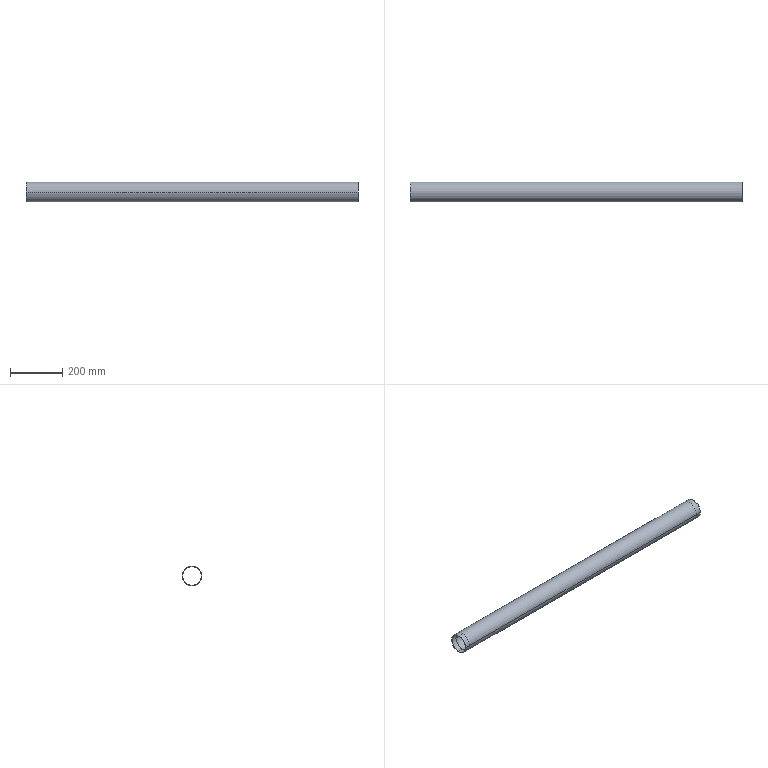Part | STEP file | DCV-000-001 | 1 solid | 12 faces | box 1270 x 76.3 x 76.3 mm | volume 923470 mm3 | cylinder 8 | plane 4 | commonest cylinder face diameters 72 x4 69.9 x2 76.3 x2
STEP:
#1=CARTESIAN_POINT('',(0.,0.,0.));
#2=DIRECTION('',(0.,0.,1.));
#3=DIRECTION('',(1.,0.,0.));
#4=AXIS2_PLACEMENT_3D('',#1,#2,#3);
#5=CARTESIAN_POINT('',(-635.,0.,36.));
#6=VERTEX_POINT('',#5);
#7=CARTESIAN_POINT('',(-614.,0.,36.));
#8=VERTEX_POINT('',#7);
#9=CARTESIAN_POINT('',(-635.,0.,36.));
#10=DIRECTION('',(1.,0.,0.));
#11=VECTOR('',#10,1.);
#12=LINE('',#9,#11);
#13=CARTESIAN_POINT('',(-635.,0.,0.));
#14=DIRECTION('',(1.,0.,0.));
#15=DIRECTION('',(0.,0.,1.));
#16=AXIS2_PLACEMENT_3D('',#13,#14,#15);
#17=CYLINDRICAL_SURFACE('',#16,36.);
#18=CARTESIAN_POINT('',(6.283,0.));
#19=DIRECTION('',(0.,1.));
#20=VECTOR('',#19,1.);
#21=LINE('',#18,#20);
#22=(GEOMETRIC_REPRESENTATION_CONTEXT(2)PARAMETRIC_REPRESENTATION_CONTEXT()REPRESENTATION_CONTEXT('',''));
#23=DEFINITIONAL_REPRESENTATION('',(#21),#22);
#24=PCURVE('',#17,#23);
#25=CARTESIAN_POINT('',(-635.,0.,0.));
#26=DIRECTION('',(1.,0.,0.));
#27=DIRECTION('',(0.,0.,1.));
#28=AXIS2_PLACEMENT_3D('',#25,#26,#27);
#29=CYLINDRICAL_SURFACE('',#28,36.);
#30=CARTESIAN_POINT('',(0.,0.));
#31=DIRECTION('',(0.,1.));
#32=VECTOR('',#31,1.);
#33=LINE('',#30,#32);
#34=(GEOMETRIC_REPRESENTATION_CONTEXT(2)PARAMETRIC_REPRESENTATION_CONTEXT()REPRESENTATION_CONTEXT('',''));
#35=DEFINITIONAL_REPRESENTATION('',(#33),#34);
#36=PCURVE('',#29,#35);
#37=SURFACE_CURVE('',#12,(#24,#36),.PCURVE_S1.);
#38=EDGE_CURVE('',#6,#8,#37,.T.);
#39=ORIENTED_EDGE('',*,*,#38,.T.);
#40=CARTESIAN_POINT('',(-614.,0.,-36.));
#41=VERTEX_POINT('',#40);
#42=CARTESIAN_POINT('',(-614.,0.,0.));
#43=DIRECTION('',(1.,0.,0.));
#44=DIRECTION('',(0.,0.,1.));
#45=AXIS2_PLACEMENT_3D('',#42,#43,#44);
#46=CIRCLE('',#45,36.);
#47=CARTESIAN_POINT('',(0.,21.));
#48=DIRECTION('',(1.,0.));
#49=VECTOR('',#48,1.);
#50=LINE('',#47,#49);
#51=(GEOMETRIC_REPRESENTATION_CONTEXT(2)PARAMETRIC_REPRESENTATION_CONTEXT()REPRESENTATION_CONTEXT('',''));
#52=DEFINITIONAL_REPRESENTATION('',(#50),#51);
#53=PCURVE('',#17,#52);
#54=CARTESIAN_POINT('',(-614.,0.,0.));
#55=DIRECTION('',(-1.,0.,0.));
#56=DIRECTION('',(0.,0.,1.));
#57=AXIS2_PLACEMENT_3D('',#54,#55,#56);
#58=PLANE('',#57);
#59=CARTESIAN_POINT('',(36.,0.));
#60=CARTESIAN_POINT('',(36.,-62.354));
#61=CARTESIAN_POINT('',(-18.,-31.177));
#62=CARTESIAN_POINT('',(-72.,0.));
#63=CARTESIAN_POINT('',(-18.,31.177));
#64=CARTESIAN_POINT('',(36.,62.354));
#65=CARTESIAN_POINT('',(36.,0.));
#66=(BOUNDED_CURVE()B_SPLINE_CURVE(2,(#59,#60,#61,#62,#63,#64,#65),.UNSPECIFIED.,.T.,.F.)B_SPLINE_CURVE_WITH_KNOTS((1,2,2,2,2,1),(-2.094,0.,2.094,4.189,6.283,8.378),.UNSPECIFIED.)CURVE()GEOMETRIC_REPRESENTATION_ITEM()RATIONAL_B_SPLINE_CURVE((1.,0.5,1.,0.5,1.,0.5,1.))REPRESENTATION_ITEM(''));
#67=(GEOMETRIC_REPRESENTATION_CONTEXT(2)PARAMETRIC_REPRESENTATION_CONTEXT()REPRESENTATION_CONTEXT('',''));
#68=DEFINITIONAL_REPRESENTATION('',(#66),#67);
#69=PCURVE('',#58,#68);
#70=SURFACE_CURVE('',#46,(#53,#69),.PCURVE_S1.);
#71=EDGE_CURVE('',#41,#8,#70,.T.);
#72=ORIENTED_EDGE('',*,*,#71,.F.);
#73=CARTESIAN_POINT('',(-635.,0.,-36.));
#74=VERTEX_POINT('',#73);
#75=CARTESIAN_POINT('',(-635.,0.,-36.));
#76=DIRECTION('',(1.,0.,0.));
#77=VECTOR('',#76,1.);
#78=LINE('',#75,#77);
#79=CARTESIAN_POINT('',(3.142,0.));
#80=DIRECTION('',(0.,1.));
#81=VECTOR('',#80,1.);
#82=LINE('',#79,#81);
#83=(GEOMETRIC_REPRESENTATION_CONTEXT(2)PARAMETRIC_REPRESENTATION_CONTEXT()REPRESENTATION_CONTEXT('',''));
#84=DEFINITIONAL_REPRESENTATION('',(#82),#83);
#85=PCURVE('',#17,#84);
#86=CARTESIAN_POINT('',(3.142,0.));
#87=DIRECTION('',(0.,1.));
#88=VECTOR('',#87,1.);
#89=LINE('',#86,#88);
#90=(GEOMETRIC_REPRESENTATION_CONTEXT(2)PARAMETRIC_REPRESENTATION_CONTEXT()REPRESENTATION_CONTEXT('',''));
#91=DEFINITIONAL_REPRESENTATION('',(#89),#90);
#92=PCURVE('',#29,#91);
#93=SURFACE_CURVE('',#78,(#85,#92),.PCURVE_S1.);
#94=EDGE_CURVE('',#74,#41,#93,.T.);
#95=ORIENTED_EDGE('',*,*,#94,.F.);
#96=CARTESIAN_POINT('',(-635.,0.,0.));
#97=DIRECTION('',(1.,0.,0.));
#98=DIRECTION('',(0.,0.,1.));
#99=AXIS2_PLACEMENT_3D('',#96,#97,#98);
#100=CIRCLE('',#99,36.);
#101=CARTESIAN_POINT('',(0.,0.));
#102=DIRECTION('',(1.,0.));
#103=VECTOR('',#102,1.);
#104=LINE('',#101,#103);
#105=(GEOMETRIC_REPRESENTATION_CONTEXT(2)PARAMETRIC_REPRESENTATION_CONTEXT()REPRESENTATION_CONTEXT('',''));
#106=DEFINITIONAL_REPRESENTATION('',(#104),#105);
#107=PCURVE('',#17,#106);
#108=CARTESIAN_POINT('',(-635.,0.,0.));
#109=DIRECTION('',(1.,0.,0.));
#110=DIRECTION('',(0.,1.,0.));
#111=AXIS2_PLACEMENT_3D('',#108,#109,#110);
#112=PLANE('',#111);
#113=CARTESIAN_POINT('',(0.,0.));
#114=DIRECTION('',(0.,1.));
#115=AXIS2_PLACEMENT_2D('',#113,#114);
#116=CIRCLE('',#115,36.);
#117=(GEOMETRIC_REPRESENTATION_CONTEXT(2)PARAMETRIC_REPRESENTATION_CONTEXT()REPRESENTATION_CONTEXT('',''));
#118=DEFINITIONAL_REPRESENTATION('',(#116),#117);
#119=PCURVE('',#112,#118);
#120=SURFACE_CURVE('',#100,(#107,#119),.PCURVE_S1.);
#121=EDGE_CURVE('',#74,#6,#120,.T.);
#122=ORIENTED_EDGE('',*,*,#121,.T.);
#123=EDGE_LOOP('',(#39,#72,#95,#122));
#124=FACE_BOUND('',#123,.F.);
#125=ADVANCED_FACE('',(#124),#17,.F.);
#126=CARTESIAN_POINT('',(635.,0.,-36.));
#127=VERTEX_POINT('',#126);
#128=CARTESIAN_POINT('',(614.,0.,-36.));
#129=VERTEX_POINT('',#128);
#130=CARTESIAN_POINT('',(635.,0.,-36.));
#131=DIRECTION('',(-1.,0.,0.));
#132=VECTOR('',#131,1.);
#133=LINE('',#130,#132);
#134=CARTESIAN_POINT('',(635.,0.,0.));
#135=DIRECTION('',(-1.,0.,0.));
#136=DIRECTION('',(0.,0.,-1.));
#137=AXIS2_PLACEMENT_3D('',#134,#135,#136);
#138=CYLINDRICAL_SURFACE('',#137,36.);
#139=CARTESIAN_POINT('',(6.283,0.));
#140=DIRECTION('',(0.,1.));
#141=VECTOR('',#140,1.);
#142=LINE('',#139,#141);
#143=(GEOMETRIC_REPRESENTATION_CONTEXT(2)PARAMETRIC_REPRESENTATION_CONTEXT()REPRESENTATION_CONTEXT('',''));
#144=DEFINITIONAL_REPRESENTATION('',(#142),#143);
#145=PCURVE('',#138,#144);
#146=CARTESIAN_POINT('',(635.,0.,0.));
#147=DIRECTION('',(-1.,0.,0.));
#148=DIRECTION('',(0.,0.,-1.));
#149=AXIS2_PLACEMENT_3D('',#146,#147,#148);
#150=CYLINDRICAL_SURFACE('',#149,36.);
#151=CARTESIAN_POINT('',(0.,0.));
#152=DIRECTION('',(0.,1.));
#153=VECTOR('',#152,1.);
#154=LINE('',#151,#153);
#155=(GEOMETRIC_REPRESENTATION_CONTEXT(2)PARAMETRIC_REPRESENTATION_CONTEXT()REPRESENTATION_CONTEXT('',''));
#156=DEFINITIONAL_REPRESENTATION('',(#154),#155);
#157=PCURVE('',#150,#156);
#158=SURFACE_CURVE('',#133,(#145,#157),.PCURVE_S1.);
#159=EDGE_CURVE('',#127,#129,#158,.T.);
#160=ORIENTED_EDGE('',*,*,#159,.T.);
#161=CARTESIAN_POINT('',(614.,0.,36.));
#162=VERTEX_POINT('',#161);
#163=CARTESIAN_POINT('',(614.,0.,0.));
#164=DIRECTION('',(-1.,0.,0.));
#165=DIRECTION('',(0.,0.,-1.));
#166=AXIS2_PLACEMENT_3D('',#163,#164,#165);
#167=CIRCLE('',#166,36.);
#168=CARTESIAN_POINT('',(0.,21.));
#169=DIRECTION('',(1.,0.));
#170=VECTOR('',#169,1.);
#171=LINE('',#168,#170);
#172=(GEOMETRIC_REPRESENTATION_CONTEXT(2)PARAMETRIC_REPRESENTATION_CONTEXT()REPRESENTATION_CONTEXT('',''));
#173=DEFINITIONAL_REPRESENTATION('',(#171),#172);
#174=PCURVE('',#138,#173);
#175=CARTESIAN_POINT('',(614.,0.,0.));
#176=DIRECTION('',(1.,0.,0.));
#177=DIRECTION('',(0.,1.,0.));
#178=AXIS2_PLACEMENT_3D('',#175,#176,#177);
#179=PLANE('',#178);
#180=CARTESIAN_POINT('',(0.,-36.));
#181=CARTESIAN_POINT('',(-62.354,-36.));
#182=CARTESIAN_POINT('',(-31.177,18.));
#183=CARTESIAN_POINT('',(0.,72.));
#184=CARTESIAN_POINT('',(31.177,18.));
#185=CARTESIAN_POINT('',(62.354,-36.));
#186=CARTESIAN_POINT('',(0.,-36.));
#187=(BOUNDED_CURVE()B_SPLINE_CURVE(2,(#180,#181,#182,#183,#184,#185,#186),.UNSPECIFIED.,.T.,.F.)B_SPLINE_CURVE_WITH_KNOTS((1,2,2,2,2,1),(-2.094,0.,2.094,4.189,6.283,8.378),.UNSPECIFIED.)CURVE()GEOMETRIC_REPRESENTATION_ITEM()RATIONAL_B_SPLINE_CURVE((1.,0.5,1.,0.5,1.,0.5,1.))REPRESENTATION_ITEM(''));
#188=(GEOMETRIC_REPRESENTATION_CONTEXT(2)PARAMETRIC_REPRESENTATION_CONTEXT()REPRESENTATION_CONTEXT('',''));
#189=DEFINITIONAL_REPRESENTATION('',(#187),#188);
#190=PCURVE('',#179,#189);
#191=SURFACE_CURVE('',#167,(#174,#190),.PCURVE_S1.);
#192=EDGE_CURVE('',#162,#129,#191,.T.);
#193=ORIENTED_EDGE('',*,*,#192,.F.);
#194=CARTESIAN_POINT('',(635.,0.,36.));
#195=VERTEX_POINT('',#194);
#196=CARTESIAN_POINT('',(635.,0.,36.));
#197=DIRECTION('',(-1.,0.,0.));
#198=VECTOR('',#197,1.);
#199=LINE('',#196,#198);
#200=CARTESIAN_POINT('',(3.142,0.));
#201=DIRECTION('',(0.,1.));
#202=VECTOR('',#201,1.);
#203=LINE('',#200,#202);
#204=(GEOMETRIC_REPRESENTATION_CONTEXT(2)PARAMETRIC_REPRESENTATION_CONTEXT()REPRESENTATION_CONTEXT('',''));
#205=DEFINITIONAL_REPRESENTATION('',(#203),#204);
#206=PCURVE('',#138,#205);
#207=CARTESIAN_POINT('',(3.142,0.));
#208=DIRECTION('',(0.,1.));
#209=VECTOR('',#208,1.);
#210=LINE('',#207,#209);
#211=(GEOMETRIC_REPRESENTATION_CONTEXT(2)PARAMETRIC_REPRESENTATION_CONTEXT()REPRESENTATION_CONTEXT('',''));
#212=DEFINITIONAL_REPRESENTATION('',(#210),#211);
#213=PCURVE('',#150,#212);
#214=SURFACE_CURVE('',#199,(#206,#213),.PCURVE_S1.);
#215=EDGE_CURVE('',#195,#162,#214,.T.);
#216=ORIENTED_EDGE('',*,*,#215,.F.);
#217=CARTESIAN_POINT('',(635.,0.,0.));
#218=DIRECTION('',(-1.,0.,0.));
#219=DIRECTION('',(0.,0.,-1.));
#220=AXIS2_PLACEMENT_3D('',#217,#218,#219);
#221=CIRCLE('',#220,36.);
#222=CARTESIAN_POINT('',(0.,0.));
#223=DIRECTION('',(1.,0.));
#224=VECTOR('',#223,1.);
#225=LINE('',#222,#224);
#226=(GEOMETRIC_REPRESENTATION_CONTEXT(2)PARAMETRIC_REPRESENTATION_CONTEXT()REPRESENTATION_CONTEXT('',''));
#227=DEFINITIONAL_REPRESENTATION('',(#225),#226);
#228=PCURVE('',#138,#227);
#229=CARTESIAN_POINT('',(635.,0.,0.));
#230=DIRECTION('',(1.,0.,0.));
#231=DIRECTION('',(0.,1.,0.));
#232=AXIS2_PLACEMENT_3D('',#229,#230,#231);
#233=PLANE('',#232);
#234=CARTESIAN_POINT('',(0.,-36.));
#235=CARTESIAN_POINT('',(-62.354,-36.));
#236=CARTESIAN_POINT('',(-31.177,18.));
#237=CARTESIAN_POINT('',(0.,72.));
#238=CARTESIAN_POINT('',(31.177,18.));
#239=CARTESIAN_POINT('',(62.354,-36.));
#240=CARTESIAN_POINT('',(0.,-36.));
#241=(BOUNDED_CURVE()B_SPLINE_CURVE(2,(#234,#235,#236,#237,#238,#239,#240),.UNSPECIFIED.,.T.,.F.)B_SPLINE_CURVE_WITH_KNOTS((1,2,2,2,2,1),(-2.094,0.,2.094,4.189,6.283,8.378),.UNSPECIFIED.)CURVE()GEOMETRIC_REPRESENTATION_ITEM()RATIONAL_B_SPLINE_CURVE((1.,0.5,1.,0.5,1.,0.5,1.))REPRESENTATION_ITEM(''));
#242=(GEOMETRIC_REPRESENTATION_CONTEXT(2)PARAMETRIC_REPRESENTATION_CONTEXT()REPRESENTATION_CONTEXT('',''));
#243=DEFINITIONAL_REPRESENTATION('',(#241),#242);
#244=PCURVE('',#233,#243);
#245=SURFACE_CURVE('',#221,(#228,#244),.PCURVE_S1.);
#246=EDGE_CURVE('',#195,#127,#245,.T.);
#247=ORIENTED_EDGE('',*,*,#246,.T.);
#248=EDGE_LOOP('',(#160,#193,#216,#247));
#249=FACE_BOUND('',#248,.F.);
#250=ADVANCED_FACE('',(#249),#138,.F.);
#251=CARTESIAN_POINT('',(-614.,-34.95,0.));
#252=VERTEX_POINT('',#251);
#253=CARTESIAN_POINT('',(614.,-34.95,0.));
#254=VERTEX_POINT('',#253);
#255=CARTESIAN_POINT('',(0.,-34.95,0.));
#256=DIRECTION('',(1.,0.,0.));
#257=VECTOR('',#256,1.);
#258=LINE('',#255,#257);
#259=CARTESIAN_POINT('',(0.,0.,0.));
#260=DIRECTION('',(1.,0.,0.));
#261=DIRECTION('',(0.,-1.,0.));
#262=AXIS2_PLACEMENT_3D('',#259,#260,#261);
#263=CYLINDRICAL_SURFACE('',#262,34.95);
#264=CARTESIAN_POINT('',(6.283,0.));
#265=DIRECTION('',(0.,1.));
#266=VECTOR('',#265,1.);
#267=LINE('',#264,#266);
#268=(GEOMETRIC_REPRESENTATION_CONTEXT(2)PARAMETRIC_REPRESENTATION_CONTEXT()REPRESENTATION_CONTEXT('',''));
#269=DEFINITIONAL_REPRESENTATION('',(#267),#268);
#270=PCURVE('',#263,#269);
#271=CARTESIAN_POINT('',(0.,0.,0.));
#272=DIRECTION('',(1.,0.,0.));
#273=DIRECTION('',(0.,-1.,0.));
#274=AXIS2_PLACEMENT_3D('',#271,#272,#273);
#275=CYLINDRICAL_SURFACE('',#274,34.95);
#276=CARTESIAN_POINT('',(0.,0.));
#277=DIRECTION('',(0.,1.));
#278=VECTOR('',#277,1.);
#279=LINE('',#276,#278);
#280=(GEOMETRIC_REPRESENTATION_CONTEXT(2)PARAMETRIC_REPRESENTATION_CONTEXT()REPRESENTATION_CONTEXT('',''));
#281=DEFINITIONAL_REPRESENTATION('',(#279),#280);
#282=PCURVE('',#275,#281);
#283=SURFACE_CURVE('',#258,(#270,#282),.PCURVE_S1.);
#284=EDGE_CURVE('',#252,#254,#283,.T.);
#285=ORIENTED_EDGE('',*,*,#284,.T.);
#286=CARTESIAN_POINT('',(614.,34.95,0.));
#287=VERTEX_POINT('',#286);
#288=CARTESIAN_POINT('',(614.,0.,0.));
#289=DIRECTION('',(1.,0.,0.));
#290=DIRECTION('',(0.,-1.,0.));
#291=AXIS2_PLACEMENT_3D('',#288,#289,#290);
#292=CIRCLE('',#291,34.95);
#293=CARTESIAN_POINT('',(0.,614.));
#294=DIRECTION('',(1.,0.));
#295=VECTOR('',#294,1.);
#296=LINE('',#293,#295);
#297=(GEOMETRIC_REPRESENTATION_CONTEXT(2)PARAMETRIC_REPRESENTATION_CONTEXT()REPRESENTATION_CONTEXT('',''));
#298=DEFINITIONAL_REPRESENTATION('',(#296),#297);
#299=PCURVE('',#263,#298);
#300=CARTESIAN_POINT('',(0.,0.));
#301=DIRECTION('',(-1.,0.));
#302=AXIS2_PLACEMENT_2D('',#300,#301);
#303=CIRCLE('',#302,34.95);
#304=(GEOMETRIC_REPRESENTATION_CONTEXT(2)PARAMETRIC_REPRESENTATION_CONTEXT()REPRESENTATION_CONTEXT('',''));
#305=DEFINITIONAL_REPRESENTATION('',(#303),#304);
#306=PCURVE('',#179,#305);
#307=SURFACE_CURVE('',#292,(#299,#306),.PCURVE_S1.);
#308=EDGE_CURVE('',#287,#254,#307,.T.);
#309=ORIENTED_EDGE('',*,*,#308,.F.);
#310=CARTESIAN_POINT('',(-614.,34.95,0.));
#311=VERTEX_POINT('',#310);
#312=CARTESIAN_POINT('',(0.,34.95,0.));
#313=DIRECTION('',(1.,0.,0.));
#314=VECTOR('',#313,1.);
#315=LINE('',#312,#314);
#316=CARTESIAN_POINT('',(3.142,0.));
#317=DIRECTION('',(0.,1.));
#318=VECTOR('',#317,1.);
#319=LINE('',#316,#318);
#320=(GEOMETRIC_REPRESENTATION_CONTEXT(2)PARAMETRIC_REPRESENTATION_CONTEXT()REPRESENTATION_CONTEXT('',''));
#321=DEFINITIONAL_REPRESENTATION('',(#319),#320);
#322=PCURVE('',#263,#321);
#323=CARTESIAN_POINT('',(3.142,0.));
#324=DIRECTION('',(0.,1.));
#325=VECTOR('',#324,1.);
#326=LINE('',#323,#325);
#327=(GEOMETRIC_REPRESENTATION_CONTEXT(2)PARAMETRIC_REPRESENTATION_CONTEXT()REPRESENTATION_CONTEXT('',''));
#328=DEFINITIONAL_REPRESENTATION('',(#326),#327);
#329=PCURVE('',#275,#328);
#330=SURFACE_CURVE('',#315,(#322,#329),.PCURVE_S1.);
#331=EDGE_CURVE('',#311,#287,#330,.T.);
#332=ORIENTED_EDGE('',*,*,#331,.F.);
#333=CARTESIAN_POINT('',(-614.,0.,0.));
#334=DIRECTION('',(-1.,0.,0.));
#335=DIRECTION('',(0.,-1.,0.));
#336=AXIS2_PLACEMENT_3D('',#333,#334,#335);
#337=CIRCLE('',#336,34.95);
#338=CARTESIAN_POINT('',(6.283,-614.));
#339=DIRECTION('',(-1.,0.));
#340=VECTOR('',#339,1.);
#341=LINE('',#338,#340);
#342=(GEOMETRIC_REPRESENTATION_CONTEXT(2)PARAMETRIC_REPRESENTATION_CONTEXT()REPRESENTATION_CONTEXT('',''));
#343=DEFINITIONAL_REPRESENTATION('',(#341),#342);
#344=PCURVE('',#263,#343);
#345=CARTESIAN_POINT('',(0.,0.));
#346=DIRECTION('',(0.,-1.));
#347=AXIS2_PLACEMENT_2D('',#345,#346);
#348=CIRCLE('',#347,34.95);
#349=(GEOMETRIC_REPRESENTATION_CONTEXT(2)PARAMETRIC_REPRESENTATION_CONTEXT()REPRESENTATION_CONTEXT('',''));
#350=DEFINITIONAL_REPRESENTATION('',(#348),#349);
#351=PCURVE('',#58,#350);
#352=SURFACE_CURVE('',#337,(#344,#351),.PCURVE_S1.);
#353=EDGE_CURVE('',#252,#311,#352,.T.);
#354=ORIENTED_EDGE('',*,*,#353,.F.);
#355=EDGE_LOOP('',(#285,#309,#332,#354));
#356=FACE_BOUND('',#355,.F.);
#357=ADVANCED_FACE('',(#356),#263,.F.);
#358=CARTESIAN_POINT('',(-635.,-38.15,0.));
#359=VERTEX_POINT('',#358);
#360=CARTESIAN_POINT('',(-635.,38.15,0.));
#361=VERTEX_POINT('',#360);
#362=CARTESIAN_POINT('',(-635.,0.,0.));
#363=DIRECTION('',(-1.,0.,0.));
#364=DIRECTION('',(0.,1.,0.));
#365=AXIS2_PLACEMENT_3D('',#362,#363,#364);
#366=CIRCLE('',#365,38.15);
#367=CARTESIAN_POINT('',(0.,0.,0.));
#368=DIRECTION('',(1.,0.,0.));
#369=DIRECTION('',(0.,1.,0.));
#370=AXIS2_PLACEMENT_3D('',#367,#368,#369);
#371=CYLINDRICAL_SURFACE('',#370,38.15);
#372=CARTESIAN_POINT('',(6.283,-635.));
#373=DIRECTION('',(-1.,0.));
#374=VECTOR('',#373,1.);
#375=LINE('',#372,#374);
#376=(GEOMETRIC_REPRESENTATION_CONTEXT(2)PARAMETRIC_REPRESENTATION_CONTEXT()REPRESENTATION_CONTEXT('',''));
#377=DEFINITIONAL_REPRESENTATION('',(#375),#376);
#378=PCURVE('',#371,#377);
#379=CARTESIAN_POINT('',(38.15,0.));
#380=CARTESIAN_POINT('',(38.15,-66.078));
#381=CARTESIAN_POINT('',(-19.075,-33.039));
#382=CARTESIAN_POINT('',(-76.3,0.));
#383=CARTESIAN_POINT('',(-19.075,33.039));
#384=CARTESIAN_POINT('',(38.15,66.078));
#385=CARTESIAN_POINT('',(38.15,0.));
#386=(BOUNDED_CURVE()B_SPLINE_CURVE(2,(#379,#380,#381,#382,#383,#384,#385),.UNSPECIFIED.,.T.,.F.)B_SPLINE_CURVE_WITH_KNOTS((1,2,2,2,2,1),(-2.094,0.,2.094,4.189,6.283,8.378),.UNSPECIFIED.)CURVE()GEOMETRIC_REPRESENTATION_ITEM()RATIONAL_B_SPLINE_CURVE((1.,0.5,1.,0.5,1.,0.5,1.))REPRESENTATION_ITEM(''));
#387=(GEOMETRIC_REPRESENTATION_CONTEXT(2)PARAMETRIC_REPRESENTATION_CONTEXT()REPRESENTATION_CONTEXT('',''));
#388=DEFINITIONAL_REPRESENTATION('',(#386),#387);
#389=PCURVE('',#112,#388);
#390=SURFACE_CURVE('',#366,(#378,#389),.PCURVE_S1.);
#391=EDGE_CURVE('',#359,#361,#390,.T.);
#392=ORIENTED_EDGE('',*,*,#391,.F.);
#393=CARTESIAN_POINT('',(635.,-38.15,0.));
#394=VERTEX_POINT('',#393);
#395=CARTESIAN_POINT('',(0.,-38.15,0.));
#396=DIRECTION('',(1.,0.,0.));
#397=VECTOR('',#396,1.);
#398=LINE('',#395,#397);
#399=CARTESIAN_POINT('',(3.142,0.));
#400=DIRECTION('',(0.,1.));
#401=VECTOR('',#400,1.);
#402=LINE('',#399,#401);
#403=(GEOMETRIC_REPRESENTATION_CONTEXT(2)PARAMETRIC_REPRESENTATION_CONTEXT()REPRESENTATION_CONTEXT('',''));
#404=DEFINITIONAL_REPRESENTATION('',(#402),#403);
#405=PCURVE('',#371,#404);
#406=CARTESIAN_POINT('',(0.,0.,0.));
#407=DIRECTION('',(1.,0.,0.));
#408=DIRECTION('',(0.,1.,0.));
#409=AXIS2_PLACEMENT_3D('',#406,#407,#408);
#410=CYLINDRICAL_SURFACE('',#409,38.15);
#411=CARTESIAN_POINT('',(3.142,0.));
#412=DIRECTION('',(0.,1.));
#413=VECTOR('',#412,1.);
#414=LINE('',#411,#413);
#415=(GEOMETRIC_REPRESENTATION_CONTEXT(2)PARAMETRIC_REPRESENTATION_CONTEXT()REPRESENTATION_CONTEXT('',''));
#416=DEFINITIONAL_REPRESENTATION('',(#414),#415);
#417=PCURVE('',#410,#416);
#418=SURFACE_CURVE('',#398,(#405,#417),.PCURVE_S1.);
#419=EDGE_CURVE('',#359,#394,#418,.T.);
#420=ORIENTED_EDGE('',*,*,#419,.T.);
#421=CARTESIAN_POINT('',(635.,38.15,0.));
#422=VERTEX_POINT('',#421);
#423=CARTESIAN_POINT('',(635.,0.,0.));
#424=DIRECTION('',(1.,0.,0.));
#425=DIRECTION('',(0.,1.,0.));
#426=AXIS2_PLACEMENT_3D('',#423,#424,#425);
#427=CIRCLE('',#426,38.15);
#428=CARTESIAN_POINT('',(0.,635.));
#429=DIRECTION('',(1.,0.));
#430=VECTOR('',#429,1.);
#431=LINE('',#428,#430);
#432=(GEOMETRIC_REPRESENTATION_CONTEXT(2)PARAMETRIC_REPRESENTATION_CONTEXT()REPRESENTATION_CONTEXT('',''));
#433=DEFINITIONAL_REPRESENTATION('',(#431),#432);
#434=PCURVE('',#371,#433);
#435=CARTESIAN_POINT('',(0.,0.));
#436=DIRECTION('',(1.,0.));
#437=AXIS2_PLACEMENT_2D('',#435,#436);
#438=CIRCLE('',#437,38.15);
#439=(GEOMETRIC_REPRESENTATION_CONTEXT(2)PARAMETRIC_REPRESENTATION_CONTEXT()REPRESENTATION_CONTEXT('',''));
#440=DEFINITIONAL_REPRESENTATION('',(#438),#439);
#441=PCURVE('',#233,#440);
#442=SURFACE_CURVE('',#427,(#434,#441),.PCURVE_S1.);
#443=EDGE_CURVE('',#422,#394,#442,.T.);
#444=ORIENTED_EDGE('',*,*,#443,.F.);
#445=CARTESIAN_POINT('',(0.,38.15,0.));
#446=DIRECTION('',(1.,0.,0.));
#447=VECTOR('',#446,1.);
#448=LINE('',#445,#447);
#449=CARTESIAN_POINT('',(0.,0.));
#450=DIRECTION('',(0.,1.));
#451=VECTOR('',#450,1.);
#452=LINE('',#449,#451);
#453=(GEOMETRIC_REPRESENTATION_CONTEXT(2)PARAMETRIC_REPRESENTATION_CONTEXT()REPRESENTATION_CONTEXT('',''));
#454=DEFINITIONAL_REPRESENTATION('',(#452),#453);
#455=PCURVE('',#371,#454);
#456=CARTESIAN_POINT('',(6.283,0.));
#457=DIRECTION('',(0.,1.));
#458=VECTOR('',#457,1.);
#459=LINE('',#456,#458);
#460=(GEOMETRIC_REPRESENTATION_CONTEXT(2)PARAMETRIC_REPRESENTATION_CONTEXT()REPRESENTATION_CONTEXT('',''));
#461=DEFINITIONAL_REPRESENTATION('',(#459),#460);
#462=PCURVE('',#410,#461);
#463=SURFACE_CURVE('',#448,(#455,#462),.PCURVE_S1.);
#464=EDGE_CURVE('',#361,#422,#463,.T.);
#465=ORIENTED_EDGE('',*,*,#464,.F.);
#466=EDGE_LOOP('',(#392,#420,#444,#465));
#467=FACE_BOUND('',#466,.T.);
#468=ADVANCED_FACE('',(#467),#371,.T.);
#469=CARTESIAN_POINT('',(635.,0.,0.));
#470=DIRECTION('',(-1.,0.,0.));
#471=DIRECTION('',(0.,0.,-1.));
#472=AXIS2_PLACEMENT_3D('',#469,#470,#471);
#473=CIRCLE('',#472,36.);
#474=CARTESIAN_POINT('',(0.,-36.));
#475=CARTESIAN_POINT('',(-62.354,-36.));
#476=CARTESIAN_POINT('',(-31.177,18.));
#477=CARTESIAN_POINT('',(0.,72.));
#478=CARTESIAN_POINT('',(31.177,18.));
#479=CARTESIAN_POINT('',(62.354,-36.));
#480=CARTESIAN_POINT('',(0.,-36.));
#481=(BOUNDED_CURVE()B_SPLINE_CURVE(2,(#474,#475,#476,#477,#478,#479,#480),.UNSPECIFIED.,.T.,.F.)B_SPLINE_CURVE_WITH_KNOTS((1,2,2,2,2,1),(-2.094,0.,2.094,4.189,6.283,8.378),.UNSPECIFIED.)CURVE()GEOMETRIC_REPRESENTATION_ITEM()RATIONAL_B_SPLINE_CURVE((1.,0.5,1.,0.5,1.,0.5,1.))REPRESENTATION_ITEM(''));
#482=(GEOMETRIC_REPRESENTATION_CONTEXT(2)PARAMETRIC_REPRESENTATION_CONTEXT()REPRESENTATION_CONTEXT('',''));
#483=DEFINITIONAL_REPRESENTATION('',(#481),#482);
#484=PCURVE('',#233,#483);
#485=CARTESIAN_POINT('',(0.,0.));
#486=DIRECTION('',(1.,0.));
#487=VECTOR('',#486,1.);
#488=LINE('',#485,#487);
#489=(GEOMETRIC_REPRESENTATION_CONTEXT(2)PARAMETRIC_REPRESENTATION_CONTEXT()REPRESENTATION_CONTEXT('',''));
#490=DEFINITIONAL_REPRESENTATION('',(#488),#489);
#491=PCURVE('',#150,#490);
#492=SURFACE_CURVE('',#473,(#484,#491),.PCURVE_S1.);
#493=EDGE_CURVE('',#127,#195,#492,.T.);
#494=ORIENTED_EDGE('',*,*,#493,.T.);
#495=ORIENTED_EDGE('',*,*,#246,.T.);
#496=EDGE_LOOP('',(#494,#495));
#497=FACE_BOUND('',#496,.T.);
#498=ORIENTED_EDGE('',*,*,#443,.T.);
#499=CARTESIAN_POINT('',(635.,0.,0.));
#500=DIRECTION('',(1.,0.,0.));
#501=DIRECTION('',(0.,1.,0.));
#502=AXIS2_PLACEMENT_3D('',#499,#500,#501);
#503=CIRCLE('',#502,38.15);
#504=CARTESIAN_POINT('',(0.,0.));
#505=DIRECTION('',(1.,0.));
#506=AXIS2_PLACEMENT_2D('',#504,#505);
#507=CIRCLE('',#506,38.15);
#508=(GEOMETRIC_REPRESENTATION_CONTEXT(2)PARAMETRIC_REPRESENTATION_CONTEXT()REPRESENTATION_CONTEXT('',''));
#509=DEFINITIONAL_REPRESENTATION('',(#507),#508);
#510=PCURVE('',#233,#509);
#511=CARTESIAN_POINT('',(0.,635.));
#512=DIRECTION('',(1.,0.));
#513=VECTOR('',#512,1.);
#514=LINE('',#511,#513);
#515=(GEOMETRIC_REPRESENTATION_CONTEXT(2)PARAMETRIC_REPRESENTATION_CONTEXT()REPRESENTATION_CONTEXT('',''));
#516=DEFINITIONAL_REPRESENTATION('',(#514),#515);
#517=PCURVE('',#410,#516);
#518=SURFACE_CURVE('',#503,(#510,#517),.PCURVE_S1.);
#519=EDGE_CURVE('',#394,#422,#518,.T.);
#520=ORIENTED_EDGE('',*,*,#519,.T.);
#521=EDGE_LOOP('',(#498,#520));
#522=FACE_BOUND('',#521,.T.);
#523=ADVANCED_FACE('',(#497,#522),#233,.T.);
#524=ORIENTED_EDGE('',*,*,#419,.F.);
#525=CARTESIAN_POINT('',(-635.,0.,0.));
#526=DIRECTION('',(-1.,0.,0.));
#527=DIRECTION('',(0.,1.,0.));
#528=AXIS2_PLACEMENT_3D('',#525,#526,#527);
#529=CIRCLE('',#528,38.15);
#530=CARTESIAN_POINT('',(6.283,-635.));
#531=DIRECTION('',(-1.,0.));
#532=VECTOR('',#531,1.);
#533=LINE('',#530,#532);
#534=(GEOMETRIC_REPRESENTATION_CONTEXT(2)PARAMETRIC_REPRESENTATION_CONTEXT()REPRESENTATION_CONTEXT('',''));
#535=DEFINITIONAL_REPRESENTATION('',(#533),#534);
#536=PCURVE('',#410,#535);
#537=CARTESIAN_POINT('',(38.15,0.));
#538=CARTESIAN_POINT('',(38.15,-66.078));
#539=CARTESIAN_POINT('',(-19.075,-33.039));
#540=CARTESIAN_POINT('',(-76.3,0.));
#541=CARTESIAN_POINT('',(-19.075,33.039));
#542=CARTESIAN_POINT('',(38.15,66.078));
#543=CARTESIAN_POINT('',(38.15,0.));
#544=(BOUNDED_CURVE()B_SPLINE_CURVE(2,(#537,#538,#539,#540,#541,#542,#543),.UNSPECIFIED.,.T.,.F.)B_SPLINE_CURVE_WITH_KNOTS((1,2,2,2,2,1),(-2.094,0.,2.094,4.189,6.283,8.378),.UNSPECIFIED.)CURVE()GEOMETRIC_REPRESENTATION_ITEM()RATIONAL_B_SPLINE_CURVE((1.,0.5,1.,0.5,1.,0.5,1.))REPRESENTATION_ITEM(''));
#545=(GEOMETRIC_REPRESENTATION_CONTEXT(2)PARAMETRIC_REPRESENTATION_CONTEXT()REPRESENTATION_CONTEXT('',''));
#546=DEFINITIONAL_REPRESENTATION('',(#544),#545);
#547=PCURVE('',#112,#546);
#548=SURFACE_CURVE('',#529,(#536,#547),.PCURVE_S1.);
#549=EDGE_CURVE('',#361,#359,#548,.T.);
#550=ORIENTED_EDGE('',*,*,#549,.F.);
#551=ORIENTED_EDGE('',*,*,#464,.T.);
#552=ORIENTED_EDGE('',*,*,#519,.F.);
#553=EDGE_LOOP('',(#524,#550,#551,#552));
#554=FACE_BOUND('',#553,.T.);
#555=ADVANCED_FACE('',(#554),#410,.T.);
#556=CARTESIAN_POINT('',(614.,0.,0.));
#557=DIRECTION('',(1.,0.,0.));
#558=DIRECTION('',(0.,-1.,0.));
#559=AXIS2_PLACEMENT_3D('',#556,#557,#558);
#560=CIRCLE('',#559,34.95);
#561=CARTESIAN_POINT('',(0.,614.));
#562=DIRECTION('',(1.,0.));
#563=VECTOR('',#562,1.);
#564=LINE('',#561,#563);
#565=(GEOMETRIC_REPRESENTATION_CONTEXT(2)PARAMETRIC_REPRESENTATION_CONTEXT()REPRESENTATION_CONTEXT('',''));
#566=DEFINITIONAL_REPRESENTATION('',(#564),#565);
#567=PCURVE('',#275,#566);
#568=CARTESIAN_POINT('',(0.,0.));
#569=DIRECTION('',(-1.,0.));
#570=AXIS2_PLACEMENT_2D('',#568,#569);
#571=CIRCLE('',#570,34.95);
#572=(GEOMETRIC_REPRESENTATION_CONTEXT(2)PARAMETRIC_REPRESENTATION_CONTEXT()REPRESENTATION_CONTEXT('',''));
#573=DEFINITIONAL_REPRESENTATION('',(#571),#572);
#574=PCURVE('',#179,#573);
#575=SURFACE_CURVE('',#560,(#567,#574),.PCURVE_S1.);
#576=EDGE_CURVE('',#254,#287,#575,.T.);
#577=ORIENTED_EDGE('',*,*,#576,.F.);
#578=ORIENTED_EDGE('',*,*,#284,.F.);
#579=CARTESIAN_POINT('',(-614.,0.,0.));
#580=DIRECTION('',(-1.,0.,0.));
#581=DIRECTION('',(0.,-1.,0.));
#582=AXIS2_PLACEMENT_3D('',#579,#580,#581);
#583=CIRCLE('',#582,34.95);
#584=CARTESIAN_POINT('',(6.283,-614.));
#585=DIRECTION('',(-1.,0.));
#586=VECTOR('',#585,1.);
#587=LINE('',#584,#586);
#588=(GEOMETRIC_REPRESENTATION_CONTEXT(2)PARAMETRIC_REPRESENTATION_CONTEXT()REPRESENTATION_CONTEXT('',''));
#589=DEFINITIONAL_REPRESENTATION('',(#587),#588);
#590=PCURVE('',#275,#589);
#591=CARTESIAN_POINT('',(0.,0.));
#592=DIRECTION('',(0.,-1.));
#593=AXIS2_PLACEMENT_2D('',#591,#592);
#594=CIRCLE('',#593,34.95);
#595=(GEOMETRIC_REPRESENTATION_CONTEXT(2)PARAMETRIC_REPRESENTATION_CONTEXT()REPRESENTATION_CONTEXT('',''));
#596=DEFINITIONAL_REPRESENTATION('',(#594),#595);
#597=PCURVE('',#58,#596);
#598=SURFACE_CURVE('',#583,(#590,#597),.PCURVE_S1.);
#599=EDGE_CURVE('',#311,#252,#598,.T.);
#600=ORIENTED_EDGE('',*,*,#599,.F.);
#601=ORIENTED_EDGE('',*,*,#331,.T.);
#602=EDGE_LOOP('',(#577,#578,#600,#601));
#603=FACE_BOUND('',#602,.F.);
#604=ADVANCED_FACE('',(#603),#275,.F.);
#605=CARTESIAN_POINT('',(-635.,0.,0.));
#606=DIRECTION('',(1.,0.,0.));
#607=DIRECTION('',(0.,0.,1.));
#608=AXIS2_PLACEMENT_3D('',#605,#606,#607);
#609=CIRCLE('',#608,36.);
#610=CARTESIAN_POINT('',(0.,0.));
#611=DIRECTION('',(0.,1.));
#612=AXIS2_PLACEMENT_2D('',#610,#611);
#613=CIRCLE('',#612,36.);
#614=(GEOMETRIC_REPRESENTATION_CONTEXT(2)PARAMETRIC_REPRESENTATION_CONTEXT()REPRESENTATION_CONTEXT('',''));
#615=DEFINITIONAL_REPRESENTATION('',(#613),#614);
#616=PCURVE('',#112,#615);
#617=CARTESIAN_POINT('',(0.,0.));
#618=DIRECTION('',(1.,0.));
#619=VECTOR('',#618,1.);
#620=LINE('',#617,#619);
#621=(GEOMETRIC_REPRESENTATION_CONTEXT(2)PARAMETRIC_REPRESENTATION_CONTEXT()REPRESENTATION_CONTEXT('',''));
#622=DEFINITIONAL_REPRESENTATION('',(#620),#621);
#623=PCURVE('',#29,#622);
#624=SURFACE_CURVE('',#609,(#616,#623),.PCURVE_S1.);
#625=EDGE_CURVE('',#6,#74,#624,.T.);
#626=ORIENTED_EDGE('',*,*,#625,.T.);
#627=ORIENTED_EDGE('',*,*,#121,.T.);
#628=EDGE_LOOP('',(#626,#627));
#629=FACE_BOUND('',#628,.T.);
#630=ORIENTED_EDGE('',*,*,#549,.T.);
#631=ORIENTED_EDGE('',*,*,#391,.T.);
#632=EDGE_LOOP('',(#630,#631));
#633=FACE_BOUND('',#632,.T.);
#634=ADVANCED_FACE('',(#629,#633),#112,.F.);
#635=ORIENTED_EDGE('',*,*,#576,.F.);
#636=ORIENTED_EDGE('',*,*,#308,.F.);
#637=EDGE_LOOP('',(#635,#636));
#638=FACE_BOUND('',#637,.T.);
#639=CARTESIAN_POINT('',(614.,0.,0.));
#640=DIRECTION('',(-1.,0.,0.));
#641=DIRECTION('',(0.,0.,-1.));
#642=AXIS2_PLACEMENT_3D('',#639,#640,#641);
#643=CIRCLE('',#642,36.);
#644=CARTESIAN_POINT('',(0.,-36.));
#645=CARTESIAN_POINT('',(-62.354,-36.));
#646=CARTESIAN_POINT('',(-31.177,18.));
#647=CARTESIAN_POINT('',(0.,72.));
#648=CARTESIAN_POINT('',(31.177,18.));
#649=CARTESIAN_POINT('',(62.354,-36.));
#650=CARTESIAN_POINT('',(0.,-36.));
#651=(BOUNDED_CURVE()B_SPLINE_CURVE(2,(#644,#645,#646,#647,#648,#649,#650),.UNSPECIFIED.,.T.,.F.)B_SPLINE_CURVE_WITH_KNOTS((1,2,2,2,2,1),(-2.094,0.,2.094,4.189,6.283,8.378),.UNSPECIFIED.)CURVE()GEOMETRIC_REPRESENTATION_ITEM()RATIONAL_B_SPLINE_CURVE((1.,0.5,1.,0.5,1.,0.5,1.))REPRESENTATION_ITEM(''));
#652=(GEOMETRIC_REPRESENTATION_CONTEXT(2)PARAMETRIC_REPRESENTATION_CONTEXT()REPRESENTATION_CONTEXT('',''));
#653=DEFINITIONAL_REPRESENTATION('',(#651),#652);
#654=PCURVE('',#179,#653);
#655=CARTESIAN_POINT('',(0.,21.));
#656=DIRECTION('',(1.,0.));
#657=VECTOR('',#656,1.);
#658=LINE('',#655,#657);
#659=(GEOMETRIC_REPRESENTATION_CONTEXT(2)PARAMETRIC_REPRESENTATION_CONTEXT()REPRESENTATION_CONTEXT('',''));
#660=DEFINITIONAL_REPRESENTATION('',(#658),#659);
#661=PCURVE('',#150,#660);
#662=SURFACE_CURVE('',#643,(#654,#661),.PCURVE_S1.);
#663=EDGE_CURVE('',#129,#162,#662,.T.);
#664=ORIENTED_EDGE('',*,*,#663,.F.);
#665=ORIENTED_EDGE('',*,*,#192,.F.);
#666=EDGE_LOOP('',(#664,#665));
#667=FACE_BOUND('',#666,.T.);
#668=ADVANCED_FACE('',(#638,#667),#179,.T.);
#669=ORIENTED_EDGE('',*,*,#663,.F.);
#670=ORIENTED_EDGE('',*,*,#159,.F.);
#671=ORIENTED_EDGE('',*,*,#493,.T.);
#672=ORIENTED_EDGE('',*,*,#215,.T.);
#673=EDGE_LOOP('',(#669,#670,#671,#672));
#674=FACE_BOUND('',#673,.F.);
#675=ADVANCED_FACE('',(#674),#150,.F.);
#676=ORIENTED_EDGE('',*,*,#353,.F.);
#677=ORIENTED_EDGE('',*,*,#599,.F.);
#678=EDGE_LOOP('',(#676,#677));
#679=FACE_BOUND('',#678,.T.);
#680=CARTESIAN_POINT('',(-614.,0.,0.));
#681=DIRECTION('',(1.,0.,0.));
#682=DIRECTION('',(0.,0.,1.));
#683=AXIS2_PLACEMENT_3D('',#680,#681,#682);
#684=CIRCLE('',#683,36.);
#685=CARTESIAN_POINT('',(36.,0.));
#686=CARTESIAN_POINT('',(36.,-62.354));
#687=CARTESIAN_POINT('',(-18.,-31.177));
#688=CARTESIAN_POINT('',(-72.,0.));
#689=CARTESIAN_POINT('',(-18.,31.177));
#690=CARTESIAN_POINT('',(36.,62.354));
#691=CARTESIAN_POINT('',(36.,0.));
#692=(BOUNDED_CURVE()B_SPLINE_CURVE(2,(#685,#686,#687,#688,#689,#690,#691),.UNSPECIFIED.,.T.,.F.)B_SPLINE_CURVE_WITH_KNOTS((1,2,2,2,2,1),(-2.094,0.,2.094,4.189,6.283,8.378),.UNSPECIFIED.)CURVE()GEOMETRIC_REPRESENTATION_ITEM()RATIONAL_B_SPLINE_CURVE((1.,0.5,1.,0.5,1.,0.5,1.))REPRESENTATION_ITEM(''));
#693=(GEOMETRIC_REPRESENTATION_CONTEXT(2)PARAMETRIC_REPRESENTATION_CONTEXT()REPRESENTATION_CONTEXT('',''));
#694=DEFINITIONAL_REPRESENTATION('',(#692),#693);
#695=PCURVE('',#58,#694);
#696=CARTESIAN_POINT('',(0.,21.));
#697=DIRECTION('',(1.,0.));
#698=VECTOR('',#697,1.);
#699=LINE('',#696,#698);
#700=(GEOMETRIC_REPRESENTATION_CONTEXT(2)PARAMETRIC_REPRESENTATION_CONTEXT()REPRESENTATION_CONTEXT('',''));
#701=DEFINITIONAL_REPRESENTATION('',(#699),#700);
#702=PCURVE('',#29,#701);
#703=SURFACE_CURVE('',#684,(#695,#702),.PCURVE_S1.);
#704=EDGE_CURVE('',#8,#41,#703,.T.);
#705=ORIENTED_EDGE('',*,*,#704,.F.);
#706=ORIENTED_EDGE('',*,*,#71,.F.);
#707=EDGE_LOOP('',(#705,#706));
#708=FACE_BOUND('',#707,.T.);
#709=ADVANCED_FACE('',(#679,#708),#58,.T.);
#710=ORIENTED_EDGE('',*,*,#704,.F.);
#711=ORIENTED_EDGE('',*,*,#38,.F.);
#712=ORIENTED_EDGE('',*,*,#625,.T.);
#713=ORIENTED_EDGE('',*,*,#94,.T.);
#714=EDGE_LOOP('',(#710,#711,#712,#713));
#715=FACE_BOUND('',#714,.F.);
#716=ADVANCED_FACE('',(#715),#29,.F.);
#717=CLOSED_SHELL('',(#125,#250,#357,#468,#523,#555,#604,#634,#668,#675,#709,#716));
#718=MANIFOLD_SOLID_BREP('',#717);
#719=(LENGTH_UNIT()NAMED_UNIT(*)SI_UNIT(.MILLI.,.METRE.));
#720=UNCERTAINTY_MEASURE_WITH_UNIT(LENGTH_MEASURE(0.0000001),#719,'','');
#721=(NAMED_UNIT(*)PLANE_ANGLE_UNIT()SI_UNIT($,.RADIAN.));
#722=(NAMED_UNIT(*)SI_UNIT($,.STERADIAN.)SOLID_ANGLE_UNIT());
#723=(GEOMETRIC_REPRESENTATION_CONTEXT(3)GLOBAL_UNCERTAINTY_ASSIGNED_CONTEXT((#720))GLOBAL_UNIT_ASSIGNED_CONTEXT((#719,#721,#722))REPRESENTATION_CONTEXT('',''));
#724=ADVANCED_BREP_SHAPE_REPRESENTATION('',(#4,#718),#723);